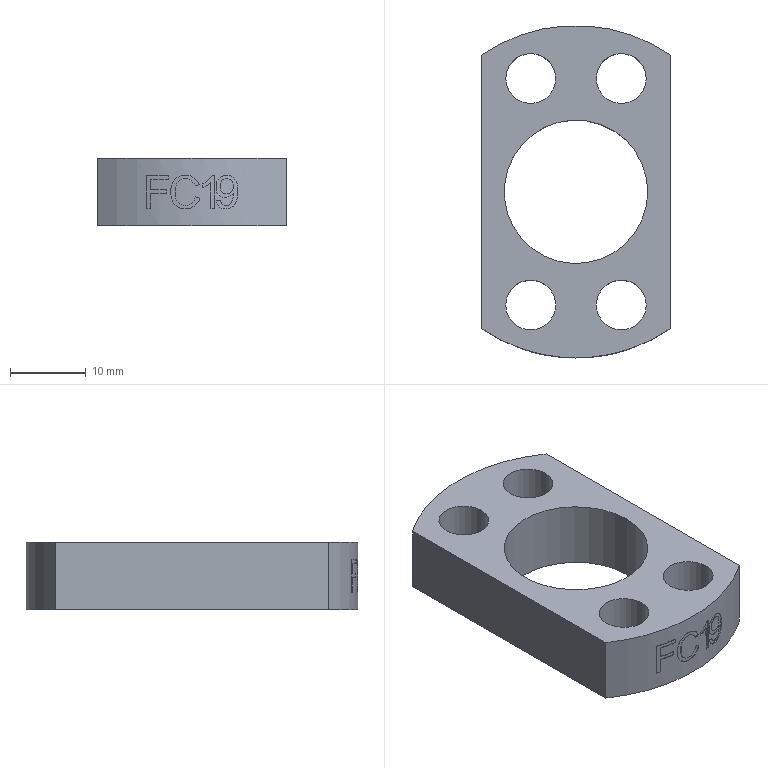Part | NX | features FC19_1 2 | 1 solid | 55 faces | box 25 x 44 x 9 mm | volume 5553 mm3 | plane 29 | cylinder 26 | commonest cylinder face diameters 6.6 x4 43.8 x4 44 x3 1.561 x1 1.724 x1 1.744 x1